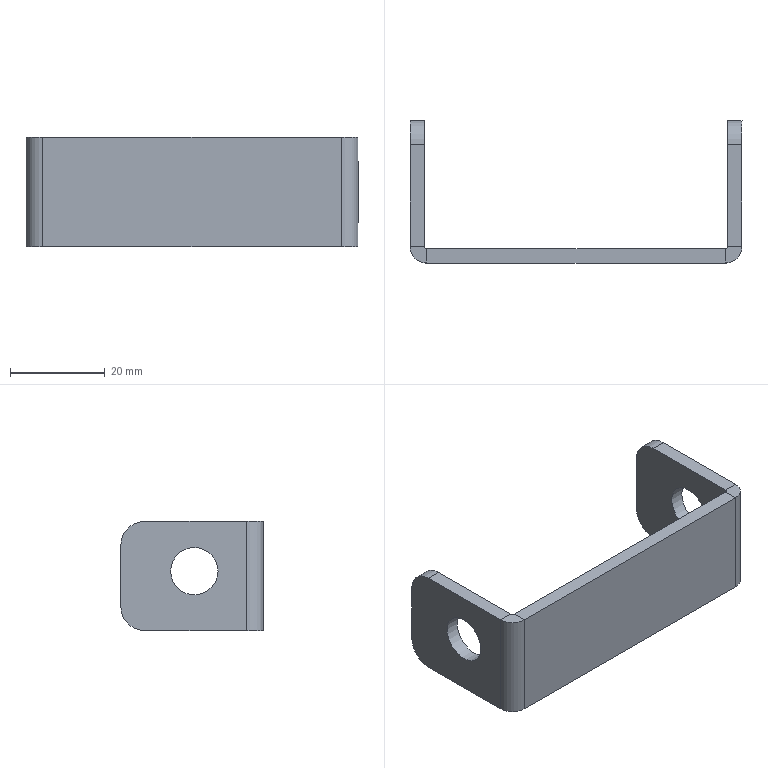Part | STEP file | Q7C0507 | 1 solid | 28 faces | box 70 x 30 x 23 mm | volume 7902 mm3 | plane 18 | cylinder 10 | commonest cylinder face diameters 10 x6 1 x2 7 x2